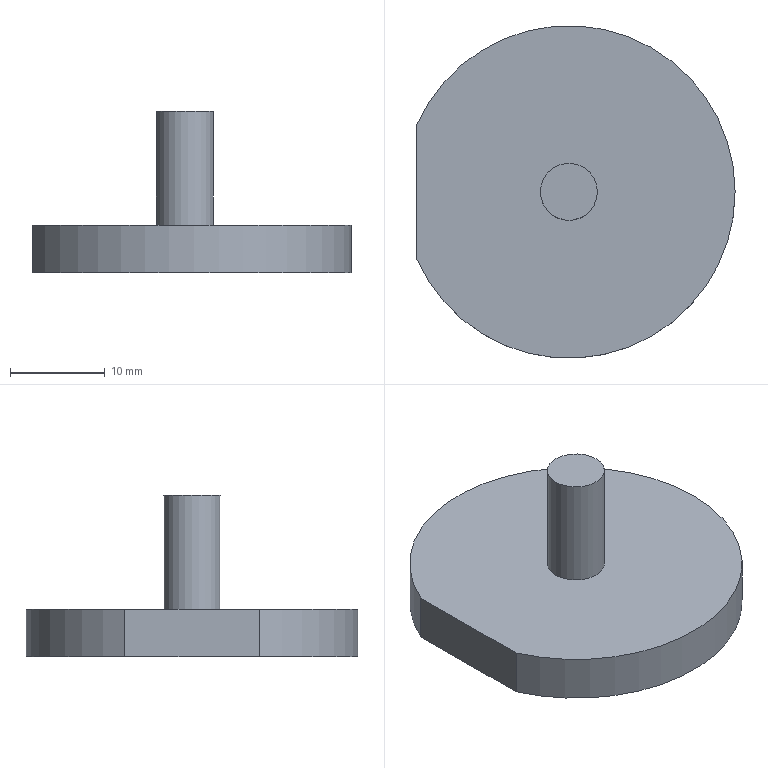Part | NX | features solid 2 | 1 solid | 6 faces | box 33.503 x 35 x 17 mm | volume 5078 mm3 | plane 4 | cylinder 2 | commonest cylinder face diameters 6 x1 35 x1
STEP:
#1=CARTESIAN_POINT('',(-409.175,-152.95,112.495));
#2=VERTEX_POINT('',#1);
#3=CARTESIAN_POINT('',(-412.175,-152.95,112.495));
#4=DIRECTION('',(0.,0.,1.));
#5=DIRECTION('',(1.,0.,0.));
#6=AXIS2_PLACEMENT_3D('',#3,#4,#5);
#7=CIRCLE('',#6,3.);
#8=EDGE_CURVE('',#2,#2,#7,.T.);
#9=ORIENTED_EDGE('',*,*,#8,.F.);
#10=EDGE_LOOP('',(#9));
#11=FACE_BOUND('',#10,.T.);
#12=CARTESIAN_POINT('',(-428.172,-160.045,112.495));
#13=VERTEX_POINT('',#12);
#14=CARTESIAN_POINT('',(-428.178,-145.867,112.495));
#15=VERTEX_POINT('',#14);
#16=CARTESIAN_POINT('',(-428.175,-152.956,112.495));
#17=DIRECTION('',(-0.000407,1.,0.));
#18=VECTOR('',#17,1000.);
#19=LINE('',#16,#18);
#20=EDGE_CURVE('',#13,#15,#19,.T.);
#21=ORIENTED_EDGE('',*,*,#20,.F.);
#22=CARTESIAN_POINT('',(-412.175,-152.95,112.495));
#23=DIRECTION('',(0.,0.,-1.));
#24=DIRECTION('',(-1.,-0.000407,0.));
#25=AXIS2_PLACEMENT_3D('',#22,#23,#24);
#26=CIRCLE('',#25,17.5);
#27=EDGE_CURVE('',#15,#13,#26,.T.);
#28=ORIENTED_EDGE('',*,*,#27,.F.);
#29=EDGE_LOOP('',(#21,#28));
#30=FACE_BOUND('',#29,.T.);
#31=CARTESIAN_POINT('',(-412.175,-152.95,112.495));
#32=DIRECTION('',(0.,0.,1.));
#33=DIRECTION('',(1.,0.000407,0.));
#34=AXIS2_PLACEMENT_3D('',#31,#32,#33);
#35=PLANE('',#34);
#36=ADVANCED_FACE('',(#11,#30),#35,.T.);
#37=CARTESIAN_POINT('',(-428.172,-160.045,107.495));
#38=VERTEX_POINT('',#37);
#39=CARTESIAN_POINT('',(-428.178,-145.867,107.495));
#40=VERTEX_POINT('',#39);
#41=CARTESIAN_POINT('',(-428.189,-118.956,107.495));
#42=DIRECTION('',(-0.000407,1.,0.));
#43=VECTOR('',#42,1000.);
#44=LINE('',#41,#43);
#45=EDGE_CURVE('',#38,#40,#44,.T.);
#46=ORIENTED_EDGE('',*,*,#45,.T.);
#47=CARTESIAN_POINT('',(-412.175,-152.95,107.495));
#48=DIRECTION('',(0.,0.,1.));
#49=DIRECTION('',(1.,0.000407,0.));
#50=AXIS2_PLACEMENT_3D('',#47,#48,#49);
#51=CIRCLE('',#50,17.5);
#52=EDGE_CURVE('',#38,#40,#51,.T.);
#53=ORIENTED_EDGE('',*,*,#52,.F.);
#54=EDGE_LOOP('',(#46,#53));
#55=FACE_BOUND('',#54,.T.);
#56=CARTESIAN_POINT('',(-412.175,-152.95,107.495));
#57=DIRECTION('',(0.,0.,-1.));
#58=DIRECTION('',(-1.,-0.000407,0.));
#59=AXIS2_PLACEMENT_3D('',#56,#57,#58);
#60=PLANE('',#59);
#61=ADVANCED_FACE('',(#55),#60,.T.);
#62=CARTESIAN_POINT('',(-428.178,-145.867,107.495));
#63=DIRECTION('',(0.,0.,1.));
#64=VECTOR('',#63,1000.);
#65=LINE('',#62,#64);
#66=EDGE_CURVE('',#15,#40,#65,.F.);
#67=ORIENTED_EDGE('',*,*,#66,.F.);
#68=ORIENTED_EDGE('',*,*,#27,.T.);
#69=CARTESIAN_POINT('',(-428.172,-160.045,107.495));
#70=DIRECTION('',(0.,0.,1.));
#71=VECTOR('',#70,1000.);
#72=LINE('',#69,#71);
#73=EDGE_CURVE('',#38,#13,#72,.T.);
#74=ORIENTED_EDGE('',*,*,#73,.F.);
#75=ORIENTED_EDGE('',*,*,#52,.T.);
#76=EDGE_LOOP('',(#67,#68,#74,#75));
#77=FACE_BOUND('',#76,.T.);
#78=CARTESIAN_POINT('',(-412.175,-152.95,107.495));
#79=DIRECTION('',(0.,0.,1.));
#80=DIRECTION('',(1.,0.000407,0.));
#81=AXIS2_PLACEMENT_3D('',#78,#79,#80);
#82=CYLINDRICAL_SURFACE('',#81,17.5);
#83=ADVANCED_FACE('',(#77),#82,.T.);
#84=ORIENTED_EDGE('',*,*,#66,.T.);
#85=ORIENTED_EDGE('',*,*,#45,.F.);
#86=ORIENTED_EDGE('',*,*,#73,.T.);
#87=ORIENTED_EDGE('',*,*,#20,.T.);
#88=EDGE_LOOP('',(#84,#85,#86,#87));
#89=FACE_BOUND('',#88,.T.);
#90=CARTESIAN_POINT('',(-428.189,-118.956,107.495));
#91=DIRECTION('',(1.,0.000407,0.));
#92=DIRECTION('',(0.,0.,-1.));
#93=AXIS2_PLACEMENT_3D('',#90,#91,#92);
#94=PLANE('',#93);
#95=ADVANCED_FACE('',(#89),#94,.F.);
#96=CARTESIAN_POINT('',(-415.175,-152.951,124.495));
#97=VERTEX_POINT('',#96);
#98=CARTESIAN_POINT('',(-412.175,-152.95,124.495));
#99=DIRECTION('',(0.,0.,-1.));
#100=DIRECTION('',(-1.,-0.000407,0.));
#101=AXIS2_PLACEMENT_3D('',#98,#99,#100);
#102=CIRCLE('',#101,3.);
#103=EDGE_CURVE('',#97,#97,#102,.T.);
#104=ORIENTED_EDGE('',*,*,#103,.F.);
#105=EDGE_LOOP('',(#104));
#106=FACE_BOUND('',#105,.T.);
#107=CARTESIAN_POINT('',(-412.175,-152.95,124.495));
#108=DIRECTION('',(0.,0.,1.));
#109=DIRECTION('',(1.,0.000407,0.));
#110=AXIS2_PLACEMENT_3D('',#107,#108,#109);
#111=PLANE('',#110);
#112=ADVANCED_FACE('',(#106),#111,.T.);
#113=ORIENTED_EDGE('',*,*,#103,.T.);
#114=EDGE_LOOP('',(#113));
#115=FACE_BOUND('',#114,.T.);
#116=ORIENTED_EDGE('',*,*,#8,.T.);
#117=EDGE_LOOP('',(#116));
#118=FACE_BOUND('',#117,.T.);
#119=CARTESIAN_POINT('',(-412.175,-152.95,112.495));
#120=DIRECTION('',(0.,0.,1.));
#121=DIRECTION('',(1.,0.000407,0.));
#122=AXIS2_PLACEMENT_3D('',#119,#120,#121);
#123=CYLINDRICAL_SURFACE('',#122,3.);
#124=ADVANCED_FACE('',(#115,#118),#123,.T.);
#125=CLOSED_SHELL('',(#36,#61,#83,#95,#112,#124));
#126=MANIFOLD_SOLID_BREP('',#125);
#127=(LENGTH_UNIT()NAMED_UNIT(*)SI_UNIT(.MILLI.,.METRE.));
#128=UNCERTAINTY_MEASURE_WITH_UNIT(LENGTH_MEASURE(0.00001),#127,'','');
#129=(NAMED_UNIT(*)PLANE_ANGLE_UNIT()SI_UNIT($,.RADIAN.));
#130=(NAMED_UNIT(*)SI_UNIT($,.STERADIAN.)SOLID_ANGLE_UNIT());
#131=(GEOMETRIC_REPRESENTATION_CONTEXT(3)GLOBAL_UNCERTAINTY_ASSIGNED_CONTEXT((#128))GLOBAL_UNIT_ASSIGNED_CONTEXT((#127,#129,#130))REPRESENTATION_CONTEXT('',''));
#132=ADVANCED_BREP_SHAPE_REPRESENTATION('',(#126),#131);